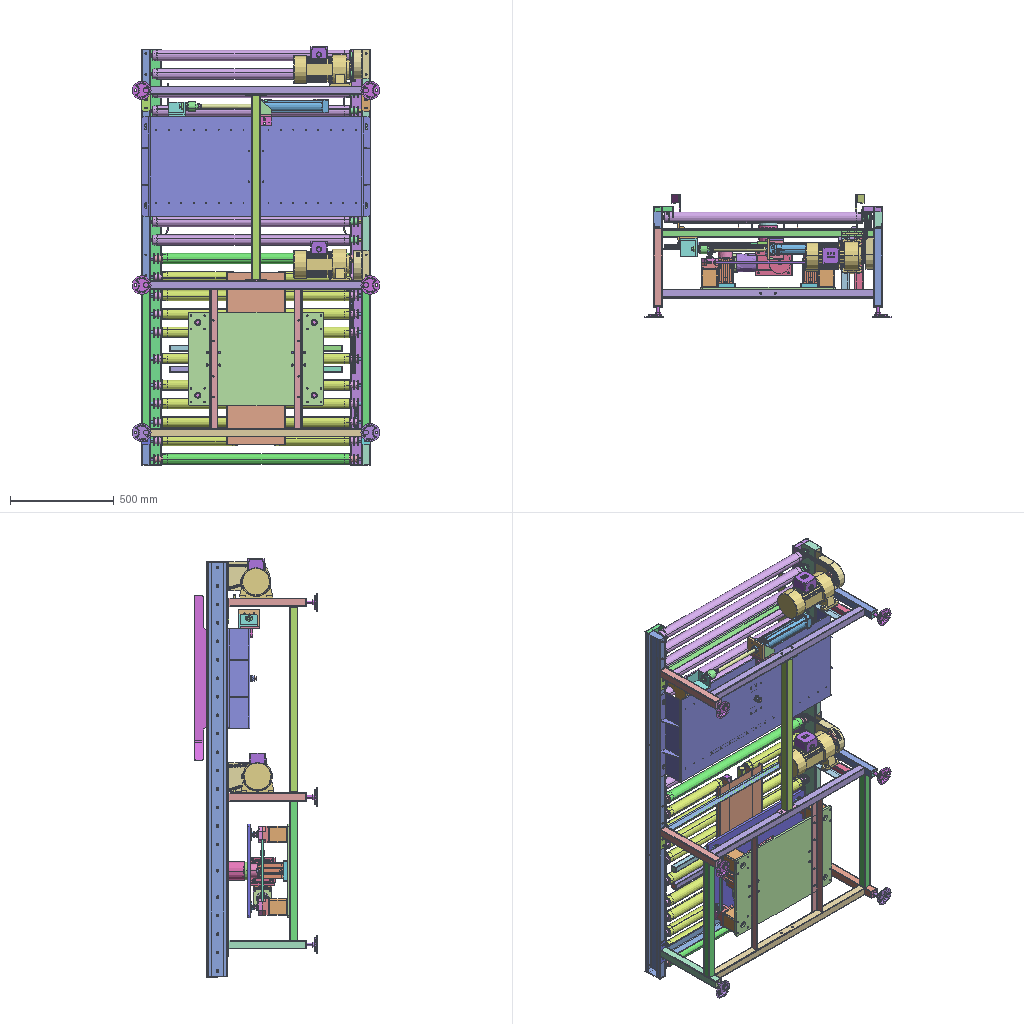Assembly | SolidWorks | 135 different items | 517 placed | box 1190 x 590 x 2017 mm
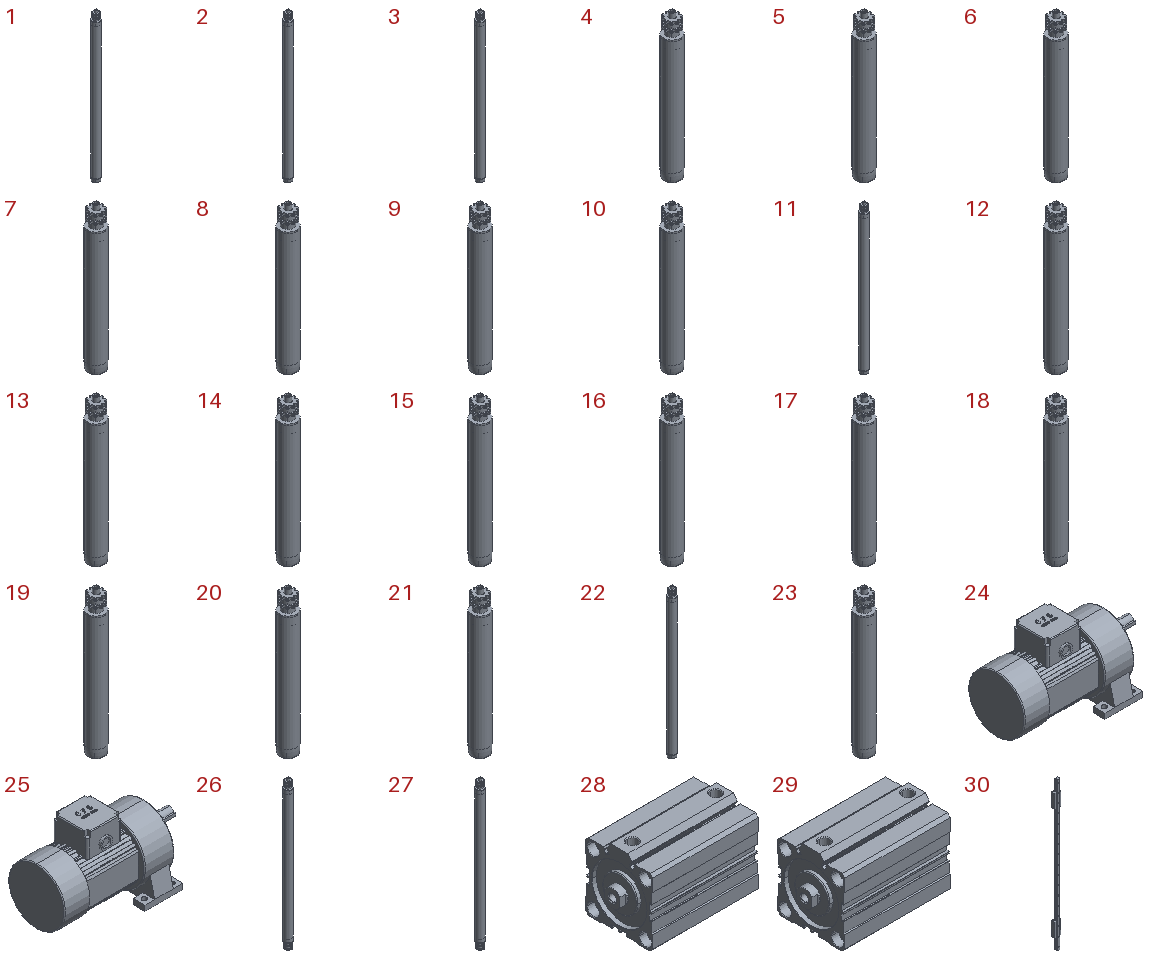Parts list (item | name | quantity | parent item | size | volume | features):
1 | (subassembly) | x1 | - | 50 x 50 x 1020 mm | 431386 mm3 | -
2 | (subassembly) | x1 | - | 50 x 50 x 1020 mm | 431386 mm3 | -
3 | (subassembly) | x1 | - | 50 x 50 x 1020 mm | 431386 mm3 | -
4 | (subassembly) | x1 | - | 50 x 50 x 432 mm | 219303 mm3 | -
5 | (subassembly) | x1 | - | 50 x 50 x 432 mm | 219303 mm3 | -
6 | (subassembly) | x1 | - | 50 x 50 x 432 mm | 219303 mm3 | -
7 | (subassembly) | x1 | - | 50 x 50 x 432 mm | 219303 mm3 | -
8 | (subassembly) | x1 | - | 50 x 50 x 432 mm | 219303 mm3 | -
9 | (subassembly) | x1 | - | 50 x 50 x 432 mm | 219303 mm3 | -
10 | (subassembly) | x1 | - | 50 x 50 x 432 mm | 219303 mm3 | -
11 | (subassembly) | x1 | - | 50 x 50 x 1020 mm | 431386 mm3 | -
12 | (subassembly) | x1 | - | 50 x 50 x 432 mm | 219303 mm3 | -
13 | (subassembly) | x1 | - | 50 x 50 x 432 mm | 219303 mm3 | -
14 | (subassembly) | x1 | - | 50 x 50 x 432 mm | 219303 mm3 | -
15 | (subassembly) | x1 | - | 50 x 50 x 432 mm | 219303 mm3 | -
16 | (subassembly) | x1 | - | 50 x 50 x 432 mm | 219303 mm3 | -
17 | (subassembly) | x1 | - | 50 x 50 x 432 mm | 219303 mm3 | -
18 | (subassembly) | x1 | - | 50 x 50 x 432 mm | 219303 mm3 | -
19 | (subassembly) | x1 | - | 50 x 50 x 432 mm | 219303 mm3 | -
20 | (subassembly) | x1 | - | 50 x 50 x 432 mm | 219303 mm3 | -
21 | (subassembly) | x1 | - | 50 x 50 x 432 mm | 219303 mm3 | -
22 | (subassembly) | x1 | - | 50 x 50 x 1020 mm | 431386 mm3 | -
23 | (subassembly) | x1 | - | 50 x 50 x 432 mm | 219303 mm3 | -
24 | (subassembly) | x1 | - | 315 x 158 x 191 mm | 4023427 mm3 | -
25 | (subassembly) | x1 | - | 315 x 158 x 191 mm | 4023427 mm3 | -
26 | (subassembly) | x1 | - | 50 x 50 x 1020 mm | 482112 mm3 | -
27 | (subassembly) | x1 | - | 50 x 50 x 1020 mm | 482112 mm3 | -
28 | (subassembly) | x1 | - | 129 x 77 x 84 mm | 432109 mm3 | -
29 | (subassembly) | x1 | - | 129 x 77 x 84 mm | 432109 mm3 | -
30 | (subassembly) | x1 | in 38 | 44 x 30 x 1000 mm | 445090 mm3 | -
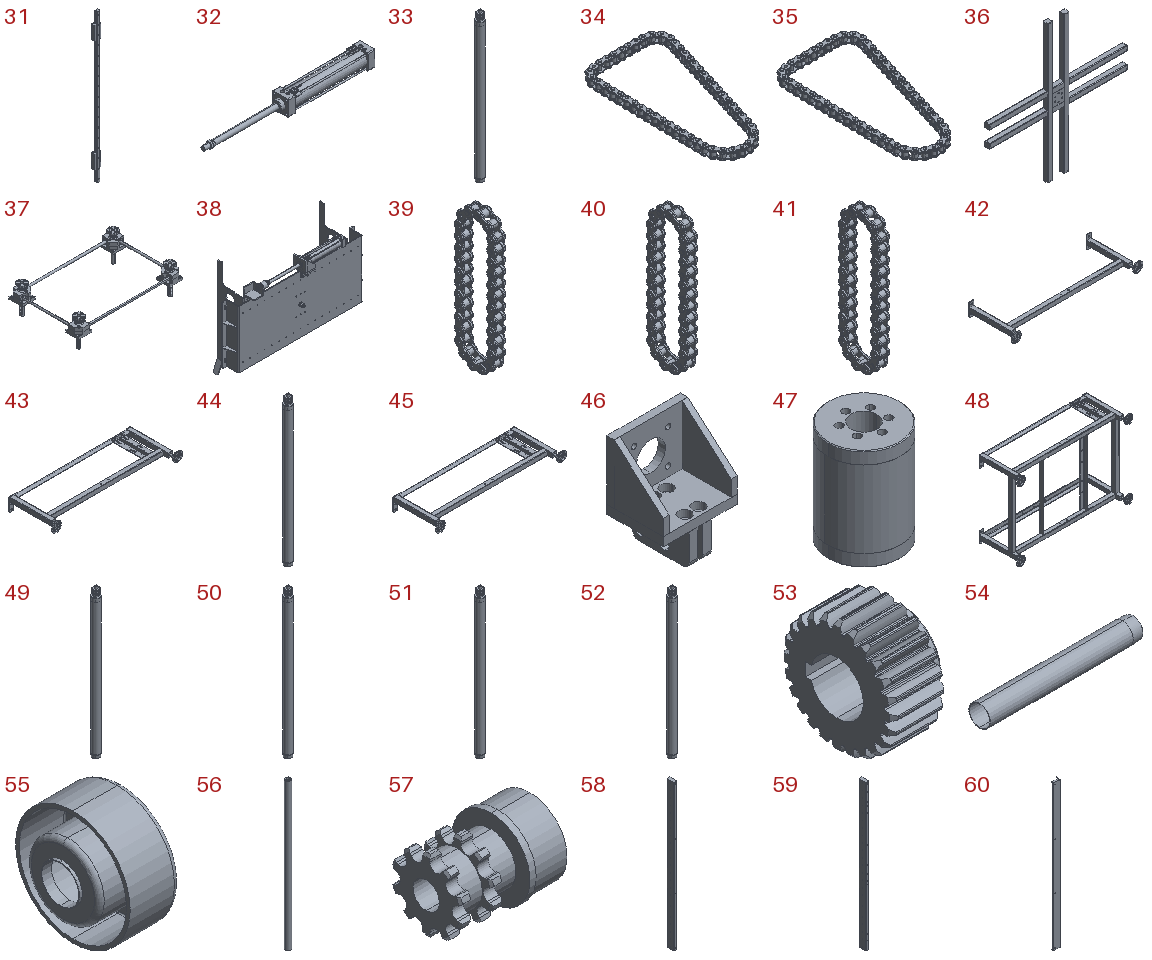31 | (subassembly) | x1 | in 38 | 44 x 30 x 1000 mm | 445090 mm3 | -
32 | (subassembly) | x1 | in 38 | 650 x 62 x 64.972 mm | 512246 mm3 | -
33 | (subassembly) | x1 | - | 50 x 50 x 1020 mm | 431386 mm3 | -
34 | (subassembly) | x1 | - | 145.929 x 266.011 x 16.575 mm | 58479 mm3 | -
35 | (subassembly) | x1 | - | 145.929 x 266.011 x 16.575 mm | 58479 mm3 | -
36 | (subassembly) | x1 | - | 830 x 30 x 830 mm | 603556 mm3 | -
37 | (subassembly) | x1 | - | - | 1356586 mm3 | -
38 | (subassembly) | x1 | - | - | 8516253 mm3 | -
39 | (subassembly) | x1 | - | 16.575 x 52.9 x 179.103 mm | 33738 mm3 | -
40 | (subassembly) | x1 | - | 16.575 x 52.9 x 179.103 mm | 33738 mm3 | -
41 | (subassembly) | x1 | - | 16.575 x 52.9 x 179.103 mm | 33738 mm3 | -
42 | (subassembly) | x1 | in 48 | 1190 x 430 x 120 mm | 533595 mm3 | -
43 | (subassembly) | x1 | - | 1190 x 430 x 145 mm | 955043 mm3 | -
44 | (subassembly) | x1 | - | 50 x 50 x 1020 mm | 431386 mm3 | -
45 | (subassembly) | x1 | in 48 | 1190 x 430 x 145 mm | 955043 mm3 | -
46 | (subassembly) | x1 | in 38 | 102 x 78 x 139 mm | 279987 mm3 | -
47 | (subassembly) | x1 | - | 89 x 89 x 125 mm | 344597 mm3 | -
48 | (subassembly) | x1 | - | 1190 x 430 x 815 mm | 2877234 mm3 | -
49 | (subassembly) | x1 | - | 50 x 50 x 1020 mm | 431386 mm3 | -
50 | (subassembly) | x1 | - | 50 x 50 x 1020 mm | 431386 mm3 | -
51 | (subassembly) | x1 | - | 50 x 50 x 1020 mm | 431386 mm3 | -
52 | (subassembly) | x1 | - | 50 x 50 x 1020 mm | 431386 mm3 | -
53 | - | x8 | in 37 | 15 x 26 x 26 mm | 4375 mm3 | features BaseBody 1
54 | - | x18 | in 4, 5, 6, 7, 8, 9, 10, 12, 13, 14, 15, 16, 17, 18, 19, 20, 21, 23 | 359.5 x 50 x 50 mm | 66032 mm3 | features BaseBody 1
55 | - | x18 | in 4, 5, 6, 7, 8, 9, 10, 12, 13, 14, 15, 16, 17, 18, 19, 20, 21, 23 | 25.129 x 46.6 x 46.6 mm | 9440 mm3 | features BaseBody 1
56 | - | x18 | in 4, 5, 6, 7, 8, 9, 10, 12, 13, 14, 15, 16, 17, 18, 19, 20, 21, 23 | 15 x 15 x 432 mm | 74812 mm3 | features BaseBody 1
57 | - | x18 | in 4, 5, 6, 7, 8, 9, 10, 12, 13, 14, 15, 16, 17, 18, 19, 20, 21, 23 | 66.6 x 50 x 50 mm | 69019 mm3 | features BaseBody 1
58 | - | x1 | - | 40 x 100 x 2000 mm | 1606592 mm3 | features BaseBody 1
59 | - | x1 | - | 40 x 100 x 2000 mm | 1606592 mm3 | features BaseBody 1
60 | - | x1 | - | 95 x 51.5 x 2005 mm | 427193 mm3 | features BaseBody 1
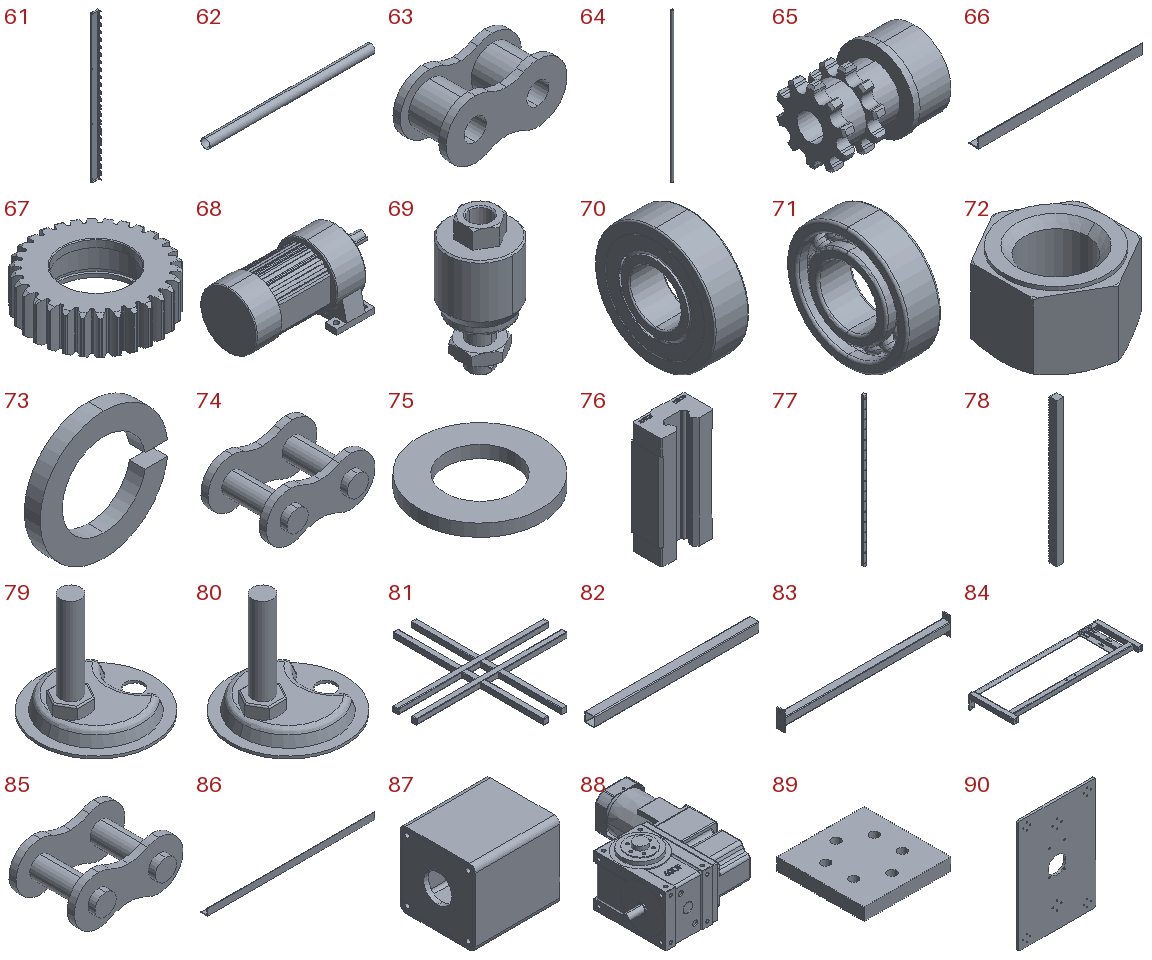61 | - | x1 | - | 95 x 51.5 x 2005 mm | 427193 mm3 | features BaseBody 1
62 | - | x2 | in 26, 27 | 898.8 x 50 x 50 mm | 165354 mm3 | features BaseBody 1
63 | - | x52 | in 34, 35 | 24.5 x 10.75 x 11.8 mm | 1261 mm3 | features BaseBody 1
64 | - | x2 | in 26, 27 | 15 x 15 x 1020 mm | 178720 mm3 | features BaseBody 1
65 | - | x4 | in 26, 27 | 66.6 x 50 x 50 mm | 69019 mm3 | features BaseBody 1
66 | - | x2 | in 48 | 670 x 40 x 40 mm | 206182 mm3 | features BaseBody 1
67 | - | x1 | in 38 | 80 x 79.651 x 25 mm | 58783 mm3 | features BaseBody 1
68 | - | x2 | in 24, 25 | 315 x 158 x 152 mm | 3662443 mm3 | features BaseBody 1
69 | - | x1 | in 38 | 44.5 x 44.5 x 90 mm | 80904 mm3 | features BaseBody 1
70 | - | x8 | in 37 | 8 x 28 x 28 mm | 3006 mm3 | features BaseBody 15
71 | - | x1 | in 38 | 15 x 52 x 52 mm | 17755 mm3 | features BaseBody 16
72 | - | x1 | in 38 | 24 x 27.713 x 16.4 mm | 5478 mm3 | features BaseBody 1
73 | - | x1 | in 38 | 25.819 x 3.2 x 25.9 mm | 926.218 mm3 | features BaseBody 1
74 | - | x45 | in 39, 40, 41 | 22.9 x 16.575 x 10.2 mm | 988.18 mm3 | features BaseBody 1
75 | - | x1 | in 38 | 30 x 30 x 3 mm | 1440 mm3 | features BaseBody 1
76 | - | x4 | in 30, 31 | 44 x 25.4 x 92.5 mm | 80377 mm3 | features BaseBody 1
77 | - | x2 | in 30, 31 | 20 x 17.5 x 1000 mm | 284337 mm3 | features BaseBody 1
78 | - | x2 | in 38 | 25 x 30 x 518.364 mm | 351700 mm3 | features BaseBody 1
79 | - | x4 | in 43, 45 | 90 x 90 x 91 mm | 39488 mm3 | features BaseBody 1
80 | - | x2 | in 42 | 90 x 90 x 91 mm | 39488 mm3 | features BaseBody 1
81 | - | x1 | in 36 | 830 x 830 x 30 mm | 556865 mm3 | features BaseBody 16
82 | - | x2 | in 48 | 670 x 40 x 40 mm | 174108 mm3 | features BaseBody 1
83 | - | x1 | - | 897.45 x 40 x 100 mm | 238563 mm3 | features BaseBody 3
84 | - | x2 | in 43, 45 | 1100 x 380 x 140 mm | 876113 mm3 | features BaseBody 11
85 | - | x52 | in 34, 35 | 22.9 x 16.575 x 10.2 mm | 988.18 mm3 | features BaseBody 1
86 | - | x2 | in 48 | 1020 x 40 x 40 mm | 314011 mm3 | features BaseBody 1
87 | - | x4 | - | 90 x 80 x 80 mm | 127903 mm3 | features BaseBody 3
88 | - | x1 | - | - | - | features RefSurface 28, BaseBody 1
89 | - | x1 | in 36 | 70 x 70 x 10 mm | 46691 mm3 | features BaseBody 1
90 | - | x1 | - | 450 x 12 x 650 mm | 3398172 mm3 | features BaseBody 1
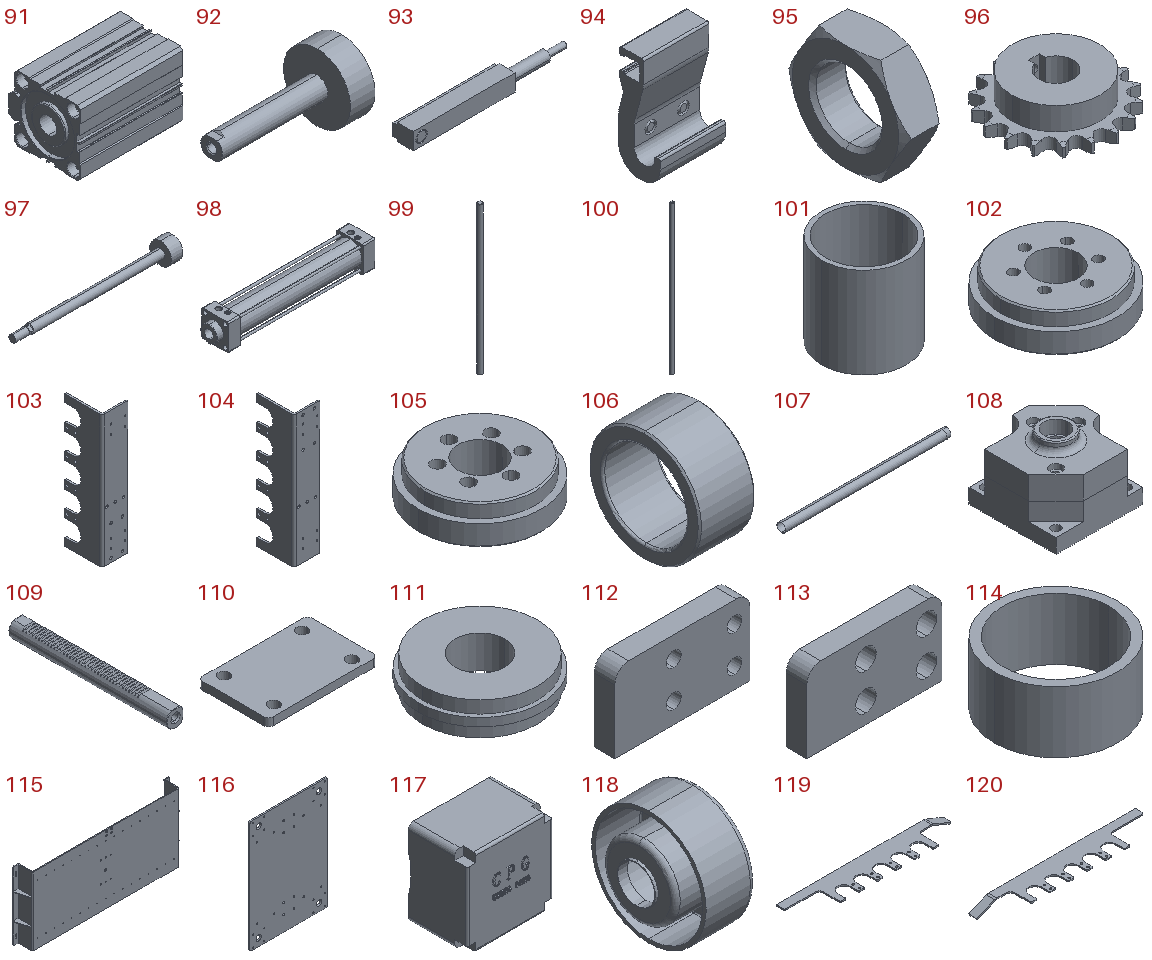91 | - | x2 | in 28, 29 | 121 x 84 x 77 mm | 331799 mm3 | features BaseBody 1
92 | - | x2 | in 28, 29 | 121.5 x 62.5 x 62.5 mm | 100309 mm3 | features BaseBody 1
93 | - | x2 | in 32 | 41.8 x 5.7 x 4.4 mm | 661.389 mm3 | features BaseBody 1
94 | - | x2 | in 32 | 18 x 13.1 x 29 mm | 2646 mm3 | features BaseBody 1
95 | - | x1 | in 32 | 8 x 26.558 x 23 mm | 2309 mm3 | features BaseBody 1
96 | - | x3 | - | 79.007 x 80 x 22 mm | 56418 mm3 | features BaseBody 1
97 | - | x1 | in 32 | 367 x 49.5 x 49.5 mm | 154752 mm3 | features BaseBody 1
98 | - | x1 | in 32 | 358 x 62 x 62 mm | 348569 mm3 | features BaseBody 1
99 | - | x2 | in 37 | 12 x 12 x 374 mm | 42082 mm3 | features BaseBody 1
100 | - | x2 | in 37 | 12 x 12 x 584 mm | 65832 mm3 | features BaseBody 1
101 | - | x1 | in 47 | 89 x 89 x 95 mm | 113486 mm3 | features BaseBody 1
102 | - | x1 | in 47 | 89 x 89 x 25 mm | 117440 mm3 | features BaseBody 1
103 | - | x1 | in 38 | 92 x 135 x 470 mm | 514041 mm3 | features BaseBody 1
104 | - | x1 | in 38 | 92 x 135 x 470 mm | 514041 mm3 | features BaseBody 1
105 | - | x1 | in 47 | 89 x 89 x 25 mm | 113670 mm3 | features BaseBody 1
106 | - | x8 | in 37 | 12 x 24 x 24 mm | 2360 mm3 | features BaseBody 1
107 | - | x11 | in 1, 2, 3, 11, 22, 33, 44, 49, 50, 51, 52 | 947.5 x 50 x 50 mm | 174207 mm3 | features BaseBody 1
108 | - | x4 | in 37 | 80 x 80 x 60 mm | 202801 mm3 | features BaseBody 4
109 | - | x4 | in 37 | 17 x 160 x 17 mm | 35318 mm3 | features BaseBody 1
110 | - | x4 | in 38 | 70 x 45 x 5 mm | 14942 mm3 | features BaseBody 1
111 | - | x8 | in 37 | 30 x 30 x 8 mm | 4203 mm3 | features BaseBody 1
112 | - | x1 | in 46 | 78 x 12 x 45 mm | 35458 mm3 | features BaseBody 1
113 | - | x1 | in 46 | 78 x 12 x 45 mm | 32787 mm3 | features BaseBody 1
114 | - | x8 | in 37 | 14 x 14 x 7 mm | 285.885 mm3 | features BaseBody 1
115 | - | x1 | in 38 | 1100 x 106 x 480 mm | 3744615 mm3 | features BaseBody 1
116 | - | x1 | - | 450 x 10 x 650 mm | 2877018 mm3 | features BaseBody 1
117 | - | x2 | in 24, 25 | 81 x 57 x 86 mm | 359652 mm3 | features BaseBody 1
118 | - | x11 | in 1, 2, 3, 11, 22, 33, 44, 49, 50, 51, 52 | 25.129 x 46.6 x 46.6 mm | 9440 mm3 | features BaseBody 1
119 | - | x1 | in 38 | 795.553 x 140 x 42.981 mm | 357455 mm3 | features BaseBody 1
120 | - | x1 | in 38 | 795.553 x 140 x 42.981 mm | 357455 mm3 | features BaseBody 1
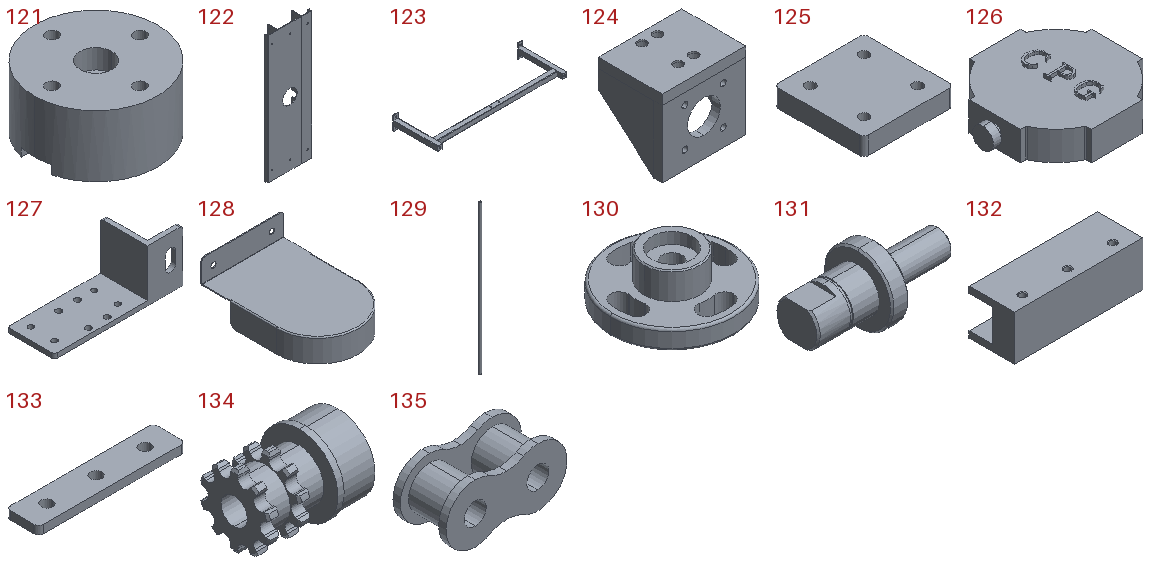121 | - | x2 | - | 70 x 70 x 35 mm | 119309 mm3 | features BaseBody 1
122 | - | x1 | - | 286 x 68 x 830 mm | 1082690 mm3 | features BaseBody 1
123 | - | x1 | in 42 | 1100 x 380 x 120 mm | 454651 mm3 | features BaseBody 7
124 | - | x1 | in 46 | 102 x 78 x 94 mm | 211743 mm3 | features BaseBody 4
125 | - | x2 | - | 100 x 100 x 20 mm | 191968 mm3 | features BaseBody 1
126 | - | x2 | in 24, 25 | 20.838 x 19 x 5 mm | 1332 mm3 | features BaseBody 1
127 | - | x1 | in 38 | 217 x 80 x 88 mm | 213969 mm3 | features BaseBody 1
128 | - | x2 | - | 140 x 200 x 78.5 mm | 67988 mm3 | features BaseBody 1
129 | - | x11 | in 1, 2, 3, 11, 22, 33, 44, 49, 50, 51, 52 | 15 x 15 x 1020 mm | 178720 mm3 | features BaseBody 1
130 | - | x4 | in 37 | 55 x 55 x 20.5 mm | 18615 mm3 | features BaseBody 1
131 | - | x1 | in 38 | 82 x 40 x 40 mm | 36185 mm3 | features BaseBody 1
132 | - | x2 | in 38 | 100 x 35 x 35 mm | 75431 mm3 | features BaseBody 1
133 | - | x2 | in 38 | 90 x 20 x 5 mm | 8384 mm3 | features BaseBody 1
134 | - | x11 | in 1, 2, 3, 11, 22, 33, 44, 49, 50, 51, 52 | 66.6 x 50 x 50 mm | 69019 mm3 | features BaseBody 1
135 | - | x45 | in 39, 40, 41 | 24.5 x 10.75 x 11.8 mm | 1261 mm3 | features BaseBody 1